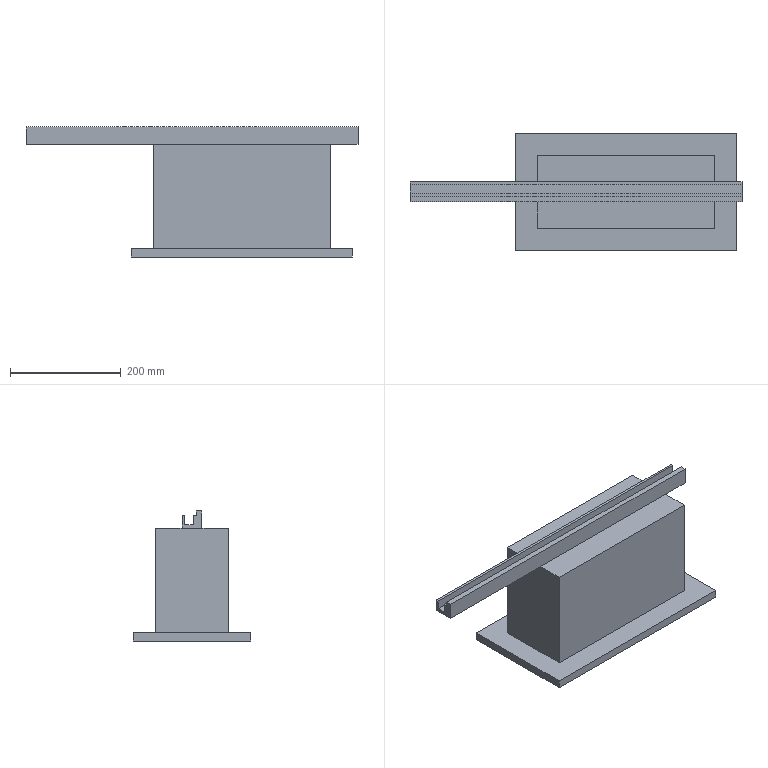Part | STEP file | CALHA_VIBRATORIA_PINO | 1 solid | 25 faces | box 600 x 212 x 235 mm | volume 9636960 mm3 | plane 25